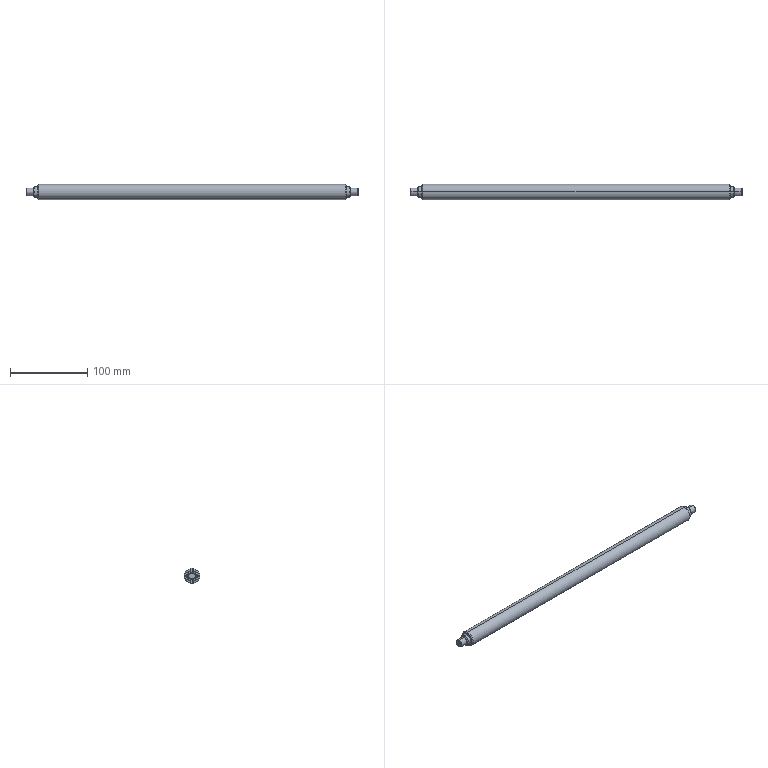Part | STEP file | Flat conveyor mechanism-CN2500x400-111-101 | 1 solid | 28 faces | box 431 x 20 x 20 mm | volume 128796 mm3 | cone 12 | cylinder 10 | plane 6 | commonest cylinder face diameters 10 x4 14 x4 20 x2
STEP:
#1=CARTESIAN_POINT('',(-200.,0.,9.));
#2=VERTEX_POINT('',#1);
#3=CARTESIAN_POINT('',(-200.,0.,-9.));
#4=VERTEX_POINT('',#3);
#5=CARTESIAN_POINT('',(-200.,0.,0.));
#6=DIRECTION('',(-1.,0.,0.));
#7=DIRECTION('',(0.,0.,-1.));
#8=AXIS2_PLACEMENT_3D('',#5,#6,#7);
#9=CIRCLE('',#8,9.);
#10=EDGE_CURVE('',#2,#4,#9,.T.);
#11=ORIENTED_EDGE('',*,*,#10,.F.);
#12=CARTESIAN_POINT('',(-199.,0.,10.));
#13=VERTEX_POINT('',#12);
#14=CARTESIAN_POINT('',(-199.,0.,10.));
#15=DIRECTION('',(0.7071,0.,0.7071));
#16=VECTOR('',#15,1000.);
#17=LINE('',#14,#16);
#18=EDGE_CURVE('',#2,#13,#17,.T.);
#19=ORIENTED_EDGE('',*,*,#18,.T.);
#20=CARTESIAN_POINT('',(-199.,0.,-10.));
#21=VERTEX_POINT('',#20);
#22=CARTESIAN_POINT('',(-199.,0.,0.));
#23=DIRECTION('',(1.,0.,0.));
#24=DIRECTION('',(0.,0.,-1.));
#25=AXIS2_PLACEMENT_3D('',#22,#23,#24);
#26=CIRCLE('',#25,10.);
#27=EDGE_CURVE('',#21,#13,#26,.T.);
#28=ORIENTED_EDGE('',*,*,#27,.F.);
#29=CARTESIAN_POINT('',(-199.,0.,-10.));
#30=DIRECTION('',(0.7071,0.,-0.7071));
#31=VECTOR('',#30,1000.);
#32=LINE('',#29,#31);
#33=EDGE_CURVE('',#4,#21,#32,.T.);
#34=ORIENTED_EDGE('',*,*,#33,.F.);
#35=EDGE_LOOP('',(#11,#19,#28,#34));
#36=FACE_OUTER_BOUND('',#35,.T.);
#37=CARTESIAN_POINT('',(-199.,0.,0.));
#38=DIRECTION('',(1.,0.,0.));
#39=DIRECTION('',(0.,0.,-1.));
#40=AXIS2_PLACEMENT_3D('',#37,#38,#39);
#41=CONICAL_SURFACE('',#40,10.,0.7854);
#42=ADVANCED_FACE('',(#36),#41,.T.);
#43=CARTESIAN_POINT('',(-215.5,0.,4.));
#44=VERTEX_POINT('',#43);
#45=CARTESIAN_POINT('',(-215.5,0.,-4.));
#46=VERTEX_POINT('',#45);
#47=CARTESIAN_POINT('',(-215.5,0.,0.));
#48=DIRECTION('',(-1.,0.,0.));
#49=DIRECTION('',(0.,0.,-1.));
#50=AXIS2_PLACEMENT_3D('',#47,#48,#49);
#51=CIRCLE('',#50,4.);
#52=EDGE_CURVE('',#44,#46,#51,.T.);
#53=ORIENTED_EDGE('',*,*,#52,.F.);
#54=CARTESIAN_POINT('',(-214.5,0.,5.));
#55=VERTEX_POINT('',#54);
#56=CARTESIAN_POINT('',(-214.5,0.,5.));
#57=DIRECTION('',(0.7071,0.,0.7071));
#58=VECTOR('',#57,1000.);
#59=LINE('',#56,#58);
#60=EDGE_CURVE('',#44,#55,#59,.T.);
#61=ORIENTED_EDGE('',*,*,#60,.T.);
#62=CARTESIAN_POINT('',(-214.5,0.,-5.));
#63=VERTEX_POINT('',#62);
#64=CARTESIAN_POINT('',(-214.5,0.,0.));
#65=DIRECTION('',(1.,0.,0.));
#66=DIRECTION('',(0.,0.,-1.));
#67=AXIS2_PLACEMENT_3D('',#64,#65,#66);
#68=CIRCLE('',#67,5.);
#69=EDGE_CURVE('',#63,#55,#68,.T.);
#70=ORIENTED_EDGE('',*,*,#69,.F.);
#71=CARTESIAN_POINT('',(-214.5,0.,-5.));
#72=DIRECTION('',(0.7071,0.,-0.7071));
#73=VECTOR('',#72,1000.);
#74=LINE('',#71,#73);
#75=EDGE_CURVE('',#46,#63,#74,.T.);
#76=ORIENTED_EDGE('',*,*,#75,.F.);
#77=EDGE_LOOP('',(#53,#61,#70,#76));
#78=FACE_OUTER_BOUND('',#77,.T.);
#79=CARTESIAN_POINT('',(-214.5,0.,0.));
#80=DIRECTION('',(1.,0.,0.));
#81=DIRECTION('',(0.,0.,-1.));
#82=AXIS2_PLACEMENT_3D('',#79,#80,#81);
#83=CONICAL_SURFACE('',#82,5.,0.7854);
#84=ADVANCED_FACE('',(#78),#83,.T.);
#85=CARTESIAN_POINT('',(200.,0.,-9.));
#86=VERTEX_POINT('',#85);
#87=CARTESIAN_POINT('',(200.,0.,9.));
#88=VERTEX_POINT('',#87);
#89=CARTESIAN_POINT('',(200.,0.,0.));
#90=DIRECTION('',(1.,0.,0.));
#91=DIRECTION('',(0.,0.,-1.));
#92=AXIS2_PLACEMENT_3D('',#89,#90,#91);
#93=CIRCLE('',#92,9.);
#94=EDGE_CURVE('',#86,#88,#93,.T.);
#95=ORIENTED_EDGE('',*,*,#94,.F.);
#96=CARTESIAN_POINT('',(199.,0.,-10.));
#97=VERTEX_POINT('',#96);
#98=CARTESIAN_POINT('',(200.,0.,-9.));
#99=DIRECTION('',(-0.7071,0.,-0.7071));
#100=VECTOR('',#99,1000.);
#101=LINE('',#98,#100);
#102=EDGE_CURVE('',#86,#97,#101,.T.);
#103=ORIENTED_EDGE('',*,*,#102,.T.);
#104=CARTESIAN_POINT('',(199.,0.,10.));
#105=VERTEX_POINT('',#104);
#106=CARTESIAN_POINT('',(199.,0.,0.));
#107=DIRECTION('',(-1.,0.,0.));
#108=DIRECTION('',(0.,0.,-1.));
#109=AXIS2_PLACEMENT_3D('',#106,#107,#108);
#110=CIRCLE('',#109,10.);
#111=EDGE_CURVE('',#105,#97,#110,.T.);
#112=ORIENTED_EDGE('',*,*,#111,.F.);
#113=CARTESIAN_POINT('',(200.,0.,9.));
#114=DIRECTION('',(-0.7071,0.,0.7071));
#115=VECTOR('',#114,1000.);
#116=LINE('',#113,#115);
#117=EDGE_CURVE('',#88,#105,#116,.T.);
#118=ORIENTED_EDGE('',*,*,#117,.F.);
#119=EDGE_LOOP('',(#95,#103,#112,#118));
#120=FACE_OUTER_BOUND('',#119,.T.);
#121=CARTESIAN_POINT('',(200.,0.,0.));
#122=DIRECTION('',(-1.,0.,0.));
#123=DIRECTION('',(0.,0.,1.));
#124=AXIS2_PLACEMENT_3D('',#121,#122,#123);
#125=CONICAL_SURFACE('',#124,9.,0.7854);
#126=ADVANCED_FACE('',(#120),#125,.T.);
#127=CARTESIAN_POINT('',(215.5,0.,-4.));
#128=VERTEX_POINT('',#127);
#129=CARTESIAN_POINT('',(215.5,0.,4.));
#130=VERTEX_POINT('',#129);
#131=CARTESIAN_POINT('',(215.5,0.,0.));
#132=DIRECTION('',(1.,0.,0.));
#133=DIRECTION('',(0.,0.,-1.));
#134=AXIS2_PLACEMENT_3D('',#131,#132,#133);
#135=CIRCLE('',#134,4.);
#136=EDGE_CURVE('',#128,#130,#135,.T.);
#137=ORIENTED_EDGE('',*,*,#136,.F.);
#138=CARTESIAN_POINT('',(214.5,0.,-5.));
#139=VERTEX_POINT('',#138);
#140=CARTESIAN_POINT('',(215.5,0.,-4.));
#141=DIRECTION('',(-0.7071,0.,-0.7071));
#142=VECTOR('',#141,1000.);
#143=LINE('',#140,#142);
#144=EDGE_CURVE('',#128,#139,#143,.T.);
#145=ORIENTED_EDGE('',*,*,#144,.T.);
#146=CARTESIAN_POINT('',(214.5,0.,5.));
#147=VERTEX_POINT('',#146);
#148=CARTESIAN_POINT('',(214.5,0.,0.));
#149=DIRECTION('',(-1.,0.,0.));
#150=DIRECTION('',(0.,0.,-1.));
#151=AXIS2_PLACEMENT_3D('',#148,#149,#150);
#152=CIRCLE('',#151,5.);
#153=EDGE_CURVE('',#147,#139,#152,.T.);
#154=ORIENTED_EDGE('',*,*,#153,.F.);
#155=CARTESIAN_POINT('',(215.5,0.,4.));
#156=DIRECTION('',(-0.7071,0.,0.7071));
#157=VECTOR('',#156,1000.);
#158=LINE('',#155,#157);
#159=EDGE_CURVE('',#130,#147,#158,.T.);
#160=ORIENTED_EDGE('',*,*,#159,.F.);
#161=EDGE_LOOP('',(#137,#145,#154,#160));
#162=FACE_OUTER_BOUND('',#161,.T.);
#163=CARTESIAN_POINT('',(215.5,0.,0.));
#164=DIRECTION('',(-1.,0.,0.));
#165=DIRECTION('',(0.,0.,1.));
#166=AXIS2_PLACEMENT_3D('',#163,#164,#165);
#167=CONICAL_SURFACE('',#166,4.,0.7854);
#168=ADVANCED_FACE('',(#162),#167,.T.);
#169=CARTESIAN_POINT('',(205.5,0.,-6.));
#170=VERTEX_POINT('',#169);
#171=CARTESIAN_POINT('',(205.5,0.,6.));
#172=VERTEX_POINT('',#171);
#173=CARTESIAN_POINT('',(205.5,0.,0.));
#174=DIRECTION('',(1.,0.,0.));
#175=DIRECTION('',(0.,0.,-1.));
#176=AXIS2_PLACEMENT_3D('',#173,#174,#175);
#177=CIRCLE('',#176,6.);
#178=EDGE_CURVE('',#170,#172,#177,.T.);
#179=ORIENTED_EDGE('',*,*,#178,.F.);
#180=CARTESIAN_POINT('',(204.5,0.,-7.));
#181=VERTEX_POINT('',#180);
#182=CARTESIAN_POINT('',(205.5,0.,-6.));
#183=DIRECTION('',(-0.7071,0.,-0.7071));
#184=VECTOR('',#183,1000.);
#185=LINE('',#182,#184);
#186=EDGE_CURVE('',#170,#181,#185,.T.);
#187=ORIENTED_EDGE('',*,*,#186,.T.);
#188=CARTESIAN_POINT('',(204.5,0.,7.));
#189=VERTEX_POINT('',#188);
#190=CARTESIAN_POINT('',(204.5,0.,0.));
#191=DIRECTION('',(-1.,0.,0.));
#192=DIRECTION('',(0.,0.,-1.));
#193=AXIS2_PLACEMENT_3D('',#190,#191,#192);
#194=CIRCLE('',#193,7.);
#195=EDGE_CURVE('',#189,#181,#194,.T.);
#196=ORIENTED_EDGE('',*,*,#195,.F.);
#197=CARTESIAN_POINT('',(205.5,0.,6.));
#198=DIRECTION('',(-0.7071,0.,0.7071));
#199=VECTOR('',#198,1000.);
#200=LINE('',#197,#199);
#201=EDGE_CURVE('',#172,#189,#200,.T.);
#202=ORIENTED_EDGE('',*,*,#201,.F.);
#203=EDGE_LOOP('',(#179,#187,#196,#202));
#204=FACE_OUTER_BOUND('',#203,.T.);
#205=CARTESIAN_POINT('',(205.5,0.,0.));
#206=DIRECTION('',(-1.,0.,0.));
#207=DIRECTION('',(0.,0.,1.));
#208=AXIS2_PLACEMENT_3D('',#205,#206,#207);
#209=CONICAL_SURFACE('',#208,6.,0.7854);
#210=ADVANCED_FACE('',(#204),#209,.T.);
#211=CARTESIAN_POINT('',(-205.5,0.,6.));
#212=VERTEX_POINT('',#211);
#213=CARTESIAN_POINT('',(-205.5,0.,-6.));
#214=VERTEX_POINT('',#213);
#215=CARTESIAN_POINT('',(-205.5,0.,0.));
#216=DIRECTION('',(-1.,0.,0.));
#217=DIRECTION('',(0.,0.,-1.));
#218=AXIS2_PLACEMENT_3D('',#215,#216,#217);
#219=CIRCLE('',#218,6.);
#220=EDGE_CURVE('',#212,#214,#219,.T.);
#221=ORIENTED_EDGE('',*,*,#220,.F.);
#222=CARTESIAN_POINT('',(-204.5,0.,7.));
#223=VERTEX_POINT('',#222);
#224=CARTESIAN_POINT('',(-204.5,0.,7.));
#225=DIRECTION('',(0.7071,0.,0.7071));
#226=VECTOR('',#225,1000.);
#227=LINE('',#224,#226);
#228=EDGE_CURVE('',#212,#223,#227,.T.);
#229=ORIENTED_EDGE('',*,*,#228,.T.);
#230=CARTESIAN_POINT('',(-204.5,0.,-7.));
#231=VERTEX_POINT('',#230);
#232=CARTESIAN_POINT('',(-204.5,0.,0.));
#233=DIRECTION('',(1.,0.,0.));
#234=DIRECTION('',(0.,0.,-1.));
#235=AXIS2_PLACEMENT_3D('',#232,#233,#234);
#236=CIRCLE('',#235,7.);
#237=EDGE_CURVE('',#231,#223,#236,.T.);
#238=ORIENTED_EDGE('',*,*,#237,.F.);
#239=CARTESIAN_POINT('',(-204.5,0.,-7.));
#240=DIRECTION('',(0.7071,0.,-0.7071));
#241=VECTOR('',#240,1000.);
#242=LINE('',#239,#241);
#243=EDGE_CURVE('',#214,#231,#242,.T.);
#244=ORIENTED_EDGE('',*,*,#243,.F.);
#245=EDGE_LOOP('',(#221,#229,#238,#244));
#246=FACE_OUTER_BOUND('',#245,.T.);
#247=CARTESIAN_POINT('',(-204.5,0.,0.));
#248=DIRECTION('',(1.,0.,0.));
#249=DIRECTION('',(0.,0.,-1.));
#250=AXIS2_PLACEMENT_3D('',#247,#248,#249);
#251=CONICAL_SURFACE('',#250,7.,0.7854);
#252=ADVANCED_FACE('',(#246),#251,.T.);
#253=ORIENTED_EDGE('',*,*,#153,.T.);
#254=CARTESIAN_POINT('',(205.5,0.,-5.));
#255=VERTEX_POINT('',#254);
#256=CARTESIAN_POINT('',(215.5,0.,-5.));
#257=DIRECTION('',(-1.,0.,0.));
#258=VECTOR('',#257,1000.);
#259=LINE('',#256,#258);
#260=EDGE_CURVE('',#139,#255,#259,.T.);
#261=ORIENTED_EDGE('',*,*,#260,.T.);
#262=CARTESIAN_POINT('',(205.5,0.,5.));
#263=VERTEX_POINT('',#262);
#264=CARTESIAN_POINT('',(205.5,0.,0.));
#265=DIRECTION('',(1.,0.,0.));
#266=DIRECTION('',(0.,0.,-1.));
#267=AXIS2_PLACEMENT_3D('',#264,#265,#266);
#268=CIRCLE('',#267,5.);
#269=EDGE_CURVE('',#255,#263,#268,.T.);
#270=ORIENTED_EDGE('',*,*,#269,.T.);
#271=CARTESIAN_POINT('',(215.5,0.,5.));
#272=DIRECTION('',(-1.,0.,0.));
#273=VECTOR('',#272,1000.);
#274=LINE('',#271,#273);
#275=EDGE_CURVE('',#147,#263,#274,.T.);
#276=ORIENTED_EDGE('',*,*,#275,.F.);
#277=EDGE_LOOP('',(#253,#261,#270,#276));
#278=FACE_OUTER_BOUND('',#277,.T.);
#279=CARTESIAN_POINT('',(215.5,0.,0.));
#280=DIRECTION('',(-1.,0.,0.));
#281=DIRECTION('',(0.,0.,1.));
#282=AXIS2_PLACEMENT_3D('',#279,#280,#281);
#283=CYLINDRICAL_SURFACE('',#282,5.);
#284=ADVANCED_FACE('',(#278),#283,.T.);
#285=CARTESIAN_POINT('',(-205.5,0.,-5.));
#286=VERTEX_POINT('',#285);
#287=CARTESIAN_POINT('',(-205.5,0.,5.));
#288=VERTEX_POINT('',#287);
#289=CARTESIAN_POINT('',(-205.5,0.,0.));
#290=DIRECTION('',(1.,0.,0.));
#291=DIRECTION('',(0.,0.,-1.));
#292=AXIS2_PLACEMENT_3D('',#289,#290,#291);
#293=CIRCLE('',#292,5.);
#294=EDGE_CURVE('',#286,#288,#293,.T.);
#295=ORIENTED_EDGE('',*,*,#294,.F.);
#296=CARTESIAN_POINT('',(215.5,0.,-5.));
#297=DIRECTION('',(-1.,0.,0.));
#298=VECTOR('',#297,1000.);
#299=LINE('',#296,#298);
#300=EDGE_CURVE('',#286,#63,#299,.T.);
#301=ORIENTED_EDGE('',*,*,#300,.T.);
#302=ORIENTED_EDGE('',*,*,#69,.T.);
#303=CARTESIAN_POINT('',(215.5,0.,5.));
#304=DIRECTION('',(-1.,0.,0.));
#305=VECTOR('',#304,1000.);
#306=LINE('',#303,#305);
#307=EDGE_CURVE('',#288,#55,#306,.T.);
#308=ORIENTED_EDGE('',*,*,#307,.F.);
#309=EDGE_LOOP('',(#295,#301,#302,#308));
#310=FACE_OUTER_BOUND('',#309,.T.);
#311=CARTESIAN_POINT('',(215.5,0.,0.));
#312=DIRECTION('',(-1.,0.,0.));
#313=DIRECTION('',(0.,0.,1.));
#314=AXIS2_PLACEMENT_3D('',#311,#312,#313);
#315=CYLINDRICAL_SURFACE('',#314,5.);
#316=ADVANCED_FACE('',(#310),#315,.T.);
#317=CARTESIAN_POINT('',(-200.,0.,7.));
#318=VERTEX_POINT('',#317);
#319=CARTESIAN_POINT('',(-200.,0.,-7.));
#320=VERTEX_POINT('',#319);
#321=CARTESIAN_POINT('',(-200.,0.,0.));
#322=DIRECTION('',(-1.,0.,0.));
#323=DIRECTION('',(0.,0.,-1.));
#324=AXIS2_PLACEMENT_3D('',#321,#322,#323);
#325=CIRCLE('',#324,7.);
#326=EDGE_CURVE('',#318,#320,#325,.T.);
#327=ORIENTED_EDGE('',*,*,#326,.T.);
#328=CARTESIAN_POINT('',(205.5,0.,-7.));
#329=DIRECTION('',(-1.,0.,0.));
#330=VECTOR('',#329,1000.);
#331=LINE('',#328,#330);
#332=EDGE_CURVE('',#320,#231,#331,.T.);
#333=ORIENTED_EDGE('',*,*,#332,.T.);
#334=ORIENTED_EDGE('',*,*,#237,.T.);
#335=CARTESIAN_POINT('',(205.5,0.,7.));
#336=DIRECTION('',(-1.,0.,0.));
#337=VECTOR('',#336,1000.);
#338=LINE('',#335,#337);
#339=EDGE_CURVE('',#318,#223,#338,.T.);
#340=ORIENTED_EDGE('',*,*,#339,.F.);
#341=EDGE_LOOP('',(#327,#333,#334,#340));
#342=FACE_OUTER_BOUND('',#341,.T.);
#343=CARTESIAN_POINT('',(205.5,0.,0.));
#344=DIRECTION('',(-1.,0.,0.));
#345=DIRECTION('',(0.,0.,1.));
#346=AXIS2_PLACEMENT_3D('',#343,#344,#345);
#347=CYLINDRICAL_SURFACE('',#346,7.);
#348=ADVANCED_FACE('',(#342),#347,.T.);
#349=ORIENTED_EDGE('',*,*,#195,.T.);
#350=CARTESIAN_POINT('',(200.,0.,-7.));
#351=VERTEX_POINT('',#350);
#352=CARTESIAN_POINT('',(205.5,0.,-7.));
#353=DIRECTION('',(-1.,0.,0.));
#354=VECTOR('',#353,1000.);
#355=LINE('',#352,#354);
#356=EDGE_CURVE('',#181,#351,#355,.T.);
#357=ORIENTED_EDGE('',*,*,#356,.T.);
#358=CARTESIAN_POINT('',(200.,0.,7.));
#359=VERTEX_POINT('',#358);
#360=CARTESIAN_POINT('',(200.,0.,0.));
#361=DIRECTION('',(-1.,0.,0.));
#362=DIRECTION('',(0.,0.,-1.));
#363=AXIS2_PLACEMENT_3D('',#360,#361,#362);
#364=CIRCLE('',#363,7.);
#365=EDGE_CURVE('',#359,#351,#364,.T.);
#366=ORIENTED_EDGE('',*,*,#365,.F.);
#367=CARTESIAN_POINT('',(205.5,0.,7.));
#368=DIRECTION('',(-1.,0.,0.));
#369=VECTOR('',#368,1000.);
#370=LINE('',#367,#369);
#371=EDGE_CURVE('',#189,#359,#370,.T.);
#372=ORIENTED_EDGE('',*,*,#371,.F.);
#373=EDGE_LOOP('',(#349,#357,#366,#372));
#374=FACE_OUTER_BOUND('',#373,.T.);
#375=CARTESIAN_POINT('',(205.5,0.,0.));
#376=DIRECTION('',(-1.,0.,0.));
#377=DIRECTION('',(0.,0.,1.));
#378=AXIS2_PLACEMENT_3D('',#375,#376,#377);
#379=CYLINDRICAL_SURFACE('',#378,7.);
#380=ADVANCED_FACE('',(#374),#379,.T.);
#381=ORIENTED_EDGE('',*,*,#111,.T.);
#382=CARTESIAN_POINT('',(200.,0.,-10.));
#383=DIRECTION('',(-1.,0.,0.));
#384=VECTOR('',#383,1000.);
#385=LINE('',#382,#384);
#386=EDGE_CURVE('',#97,#21,#385,.T.);
#387=ORIENTED_EDGE('',*,*,#386,.T.);
#388=ORIENTED_EDGE('',*,*,#27,.T.);
#389=CARTESIAN_POINT('',(200.,0.,10.));
#390=DIRECTION('',(-1.,0.,0.));
#391=VECTOR('',#390,1000.);
#392=LINE('',#389,#391);
#393=EDGE_CURVE('',#105,#13,#392,.T.);
#394=ORIENTED_EDGE('',*,*,#393,.F.);
#395=EDGE_LOOP('',(#381,#387,#388,#394));
#396=FACE_OUTER_BOUND('',#395,.T.);
#397=CARTESIAN_POINT('',(200.,0.,0.));
#398=DIRECTION('',(-1.,0.,0.));
#399=DIRECTION('',(0.,0.,1.));
#400=AXIS2_PLACEMENT_3D('',#397,#398,#399);
#401=CYLINDRICAL_SURFACE('',#400,10.);
#402=ADVANCED_FACE('',(#396),#401,.T.);
#403=ORIENTED_EDGE('',*,*,#386,.F.);
#404=CARTESIAN_POINT('',(199.,0.,0.));
#405=DIRECTION('',(-1.,0.,0.));
#406=DIRECTION('',(0.,0.,-1.));
#407=AXIS2_PLACEMENT_3D('',#404,#405,#406);
#408=CIRCLE('',#407,10.);
#409=EDGE_CURVE('',#97,#105,#408,.T.);
#410=ORIENTED_EDGE('',*,*,#409,.T.);
#411=ORIENTED_EDGE('',*,*,#393,.T.);
#412=CARTESIAN_POINT('',(-199.,0.,0.));
#413=DIRECTION('',(1.,0.,0.));
#414=DIRECTION('',(0.,0.,-1.));
#415=AXIS2_PLACEMENT_3D('',#412,#413,#414);
#416=CIRCLE('',#415,10.);
#417=EDGE_CURVE('',#13,#21,#416,.T.);
#418=ORIENTED_EDGE('',*,*,#417,.T.);
#419=EDGE_LOOP('',(#403,#410,#411,#418));
#420=FACE_OUTER_BOUND('',#419,.T.);
#421=CARTESIAN_POINT('',(200.,0.,0.));
#422=DIRECTION('',(-1.,0.,0.));
#423=DIRECTION('',(0.,0.,1.));
#424=AXIS2_PLACEMENT_3D('',#421,#422,#423);
#425=CYLINDRICAL_SURFACE('',#424,10.);
#426=ADVANCED_FACE('',(#420),#425,.T.);
#427=CARTESIAN_POINT('',(200.,0.,0.));
#428=DIRECTION('',(1.,0.,0.));
#429=DIRECTION('',(0.,0.,-1.));
#430=AXIS2_PLACEMENT_3D('',#427,#428,#429);
#431=CIRCLE('',#430,9.);
#432=EDGE_CURVE('',#88,#86,#431,.T.);
#433=ORIENTED_EDGE('',*,*,#432,.T.);
#434=ORIENTED_EDGE('',*,*,#94,.T.);
#435=EDGE_LOOP('',(#433,#434));
#436=FACE_OUTER_BOUND('',#435,.T.);
#437=ORIENTED_EDGE('',*,*,#365,.T.);
#438=CARTESIAN_POINT('',(200.,0.,0.));
#439=DIRECTION('',(-1.,0.,0.));
#440=DIRECTION('',(0.,0.,-1.));
#441=AXIS2_PLACEMENT_3D('',#438,#439,#440);
#442=CIRCLE('',#441,7.);
#443=EDGE_CURVE('',#351,#359,#442,.T.);
#444=ORIENTED_EDGE('',*,*,#443,.T.);
#445=EDGE_LOOP('',(#437,#444));
#446=FACE_BOUND('',#445,.T.);
#447=CARTESIAN_POINT('',(200.,0.,0.));
#448=DIRECTION('',(1.,0.,0.));
#449=DIRECTION('',(0.,0.,-1.));
#450=AXIS2_PLACEMENT_3D('',#447,#448,#449);
#451=PLANE('',#450);
#452=ADVANCED_FACE('',(#436,#446),#451,.T.);
#453=CARTESIAN_POINT('',(-200.,0.,0.));
#454=DIRECTION('',(-1.,0.,0.));
#455=DIRECTION('',(0.,0.,-1.));
#456=AXIS2_PLACEMENT_3D('',#453,#454,#455);
#457=CIRCLE('',#456,9.);
#458=EDGE_CURVE('',#4,#2,#457,.T.);
#459=ORIENTED_EDGE('',*,*,#458,.T.);
#460=ORIENTED_EDGE('',*,*,#10,.T.);
#461=EDGE_LOOP('',(#459,#460));
#462=FACE_OUTER_BOUND('',#461,.T.);
#463=ORIENTED_EDGE('',*,*,#326,.F.);
#464=CARTESIAN_POINT('',(-200.,0.,0.));
#465=DIRECTION('',(-1.,0.,0.));
#466=DIRECTION('',(0.,0.,-1.));
#467=AXIS2_PLACEMENT_3D('',#464,#465,#466);
#468=CIRCLE('',#467,7.);
#469=EDGE_CURVE('',#320,#318,#468,.T.);
#470=ORIENTED_EDGE('',*,*,#469,.F.);
#471=EDGE_LOOP('',(#463,#470));
#472=FACE_BOUND('',#471,.T.);
#473=CARTESIAN_POINT('',(-200.,0.,0.));
#474=DIRECTION('',(1.,0.,0.));
#475=DIRECTION('',(0.,0.,-1.));
#476=AXIS2_PLACEMENT_3D('',#473,#474,#475);
#477=PLANE('',#476);
#478=ADVANCED_FACE('',(#462,#472),#477,.F.);
#479=CARTESIAN_POINT('',(205.5,0.,0.));
#480=DIRECTION('',(1.,0.,0.));
#481=DIRECTION('',(0.,0.,-1.));
#482=AXIS2_PLACEMENT_3D('',#479,#480,#481);
#483=CIRCLE('',#482,6.);
#484=EDGE_CURVE('',#172,#170,#483,.T.);
#485=ORIENTED_EDGE('',*,*,#484,.T.);
#486=ORIENTED_EDGE('',*,*,#178,.T.);
#487=EDGE_LOOP('',(#485,#486));
#488=FACE_OUTER_BOUND('',#487,.T.);
#489=CARTESIAN_POINT('',(205.5,0.,0.));
#490=DIRECTION('',(1.,0.,0.));
#491=DIRECTION('',(0.,0.,-1.));
#492=AXIS2_PLACEMENT_3D('',#489,#490,#491);
#493=CIRCLE('',#492,5.);
#494=EDGE_CURVE('',#263,#255,#493,.T.);
#495=ORIENTED_EDGE('',*,*,#494,.F.);
#496=ORIENTED_EDGE('',*,*,#269,.F.);
#497=EDGE_LOOP('',(#495,#496));
#498=FACE_BOUND('',#497,.T.);
#499=CARTESIAN_POINT('',(205.5,0.,0.));
#500=DIRECTION('',(1.,0.,0.));
#501=DIRECTION('',(0.,0.,-1.));
#502=AXIS2_PLACEMENT_3D('',#499,#500,#501);
#503=PLANE('',#502);
#504=ADVANCED_FACE('',(#488,#498),#503,.T.);
#505=ORIENTED_EDGE('',*,*,#356,.F.);
#506=CARTESIAN_POINT('',(204.5,0.,0.));
#507=DIRECTION('',(-1.,0.,0.));
#508=DIRECTION('',(0.,0.,-1.));
#509=AXIS2_PLACEMENT_3D('',#506,#507,#508);
#510=CIRCLE('',#509,7.);
#511=EDGE_CURVE('',#181,#189,#510,.T.);
#512=ORIENTED_EDGE('',*,*,#511,.T.);
#513=ORIENTED_EDGE('',*,*,#371,.T.);
#514=ORIENTED_EDGE('',*,*,#443,.F.);
#515=EDGE_LOOP('',(#505,#512,#513,#514));
#516=FACE_OUTER_BOUND('',#515,.T.);
#517=CARTESIAN_POINT('',(205.5,0.,0.));
#518=DIRECTION('',(-1.,0.,0.));
#519=DIRECTION('',(0.,0.,1.));
#520=AXIS2_PLACEMENT_3D('',#517,#518,#519);
#521=CYLINDRICAL_SURFACE('',#520,7.);
#522=ADVANCED_FACE('',(#516),#521,.T.);
#523=ORIENTED_EDGE('',*,*,#332,.F.);
#524=ORIENTED_EDGE('',*,*,#469,.T.);
#525=ORIENTED_EDGE('',*,*,#339,.T.);
#526=CARTESIAN_POINT('',(-204.5,0.,0.));
#527=DIRECTION('',(1.,0.,0.));
#528=DIRECTION('',(0.,0.,-1.));
#529=AXIS2_PLACEMENT_3D('',#526,#527,#528);
#530=CIRCLE('',#529,7.);
#531=EDGE_CURVE('',#223,#231,#530,.T.);
#532=ORIENTED_EDGE('',*,*,#531,.T.);
#533=EDGE_LOOP('',(#523,#524,#525,#532));
#534=FACE_OUTER_BOUND('',#533,.T.);
#535=CARTESIAN_POINT('',(205.5,0.,0.));
#536=DIRECTION('',(-1.,0.,0.));
#537=DIRECTION('',(0.,0.,1.));
#538=AXIS2_PLACEMENT_3D('',#535,#536,#537);
#539=CYLINDRICAL_SURFACE('',#538,7.);
#540=ADVANCED_FACE('',(#534),#539,.T.);
#541=CARTESIAN_POINT('',(-205.5,0.,0.));
#542=DIRECTION('',(-1.,0.,0.));
#543=DIRECTION('',(0.,0.,-1.));
#544=AXIS2_PLACEMENT_3D('',#541,#542,#543);
#545=CIRCLE('',#544,6.);
#546=EDGE_CURVE('',#214,#212,#545,.T.);
#547=ORIENTED_EDGE('',*,*,#546,.T.);
#548=ORIENTED_EDGE('',*,*,#220,.T.);
#549=EDGE_LOOP('',(#547,#548));
#550=FACE_OUTER_BOUND('',#549,.T.);
#551=CARTESIAN_POINT('',(-205.5,0.,0.));
#552=DIRECTION('',(1.,0.,0.));
#553=DIRECTION('',(0.,0.,-1.));
#554=AXIS2_PLACEMENT_3D('',#551,#552,#553);
#555=CIRCLE('',#554,5.);
#556=EDGE_CURVE('',#288,#286,#555,.T.);
#557=ORIENTED_EDGE('',*,*,#556,.T.);
#558=ORIENTED_EDGE('',*,*,#294,.T.);
#559=EDGE_LOOP('',(#557,#558));
#560=FACE_BOUND('',#559,.T.);
#561=CARTESIAN_POINT('',(-205.5,0.,0.));
#562=DIRECTION('',(1.,0.,0.));
#563=DIRECTION('',(0.,0.,-1.));
#564=AXIS2_PLACEMENT_3D('',#561,#562,#563);
#565=PLANE('',#564);
#566=ADVANCED_FACE('',(#550,#560),#565,.F.);
#567=CARTESIAN_POINT('',(-215.5,0.,0.));
#568=DIRECTION('',(-1.,0.,0.));
#569=DIRECTION('',(0.,0.,-1.));
#570=AXIS2_PLACEMENT_3D('',#567,#568,#569);
#571=CIRCLE('',#570,4.);
#572=EDGE_CURVE('',#46,#44,#571,.T.);
#573=ORIENTED_EDGE('',*,*,#572,.T.);
#574=ORIENTED_EDGE('',*,*,#52,.T.);
#575=EDGE_LOOP('',(#573,#574));
#576=FACE_OUTER_BOUND('',#575,.T.);
#577=CARTESIAN_POINT('',(-215.5,0.,0.));
#578=DIRECTION('',(1.,0.,0.));
#579=DIRECTION('',(0.,0.,-1.));
#580=AXIS2_PLACEMENT_3D('',#577,#578,#579);
#581=PLANE('',#580);
#582=ADVANCED_FACE('',(#576),#581,.F.);
#583=ORIENTED_EDGE('',*,*,#300,.F.);
#584=ORIENTED_EDGE('',*,*,#556,.F.);
#585=ORIENTED_EDGE('',*,*,#307,.T.);
#586=CARTESIAN_POINT('',(-214.5,0.,0.));
#587=DIRECTION('',(1.,0.,0.));
#588=DIRECTION('',(0.,0.,-1.));
#589=AXIS2_PLACEMENT_3D('',#586,#587,#588);
#590=CIRCLE('',#589,5.);
#591=EDGE_CURVE('',#55,#63,#590,.T.);
#592=ORIENTED_EDGE('',*,*,#591,.T.);
#593=EDGE_LOOP('',(#583,#584,#585,#592));
#594=FACE_OUTER_BOUND('',#593,.T.);
#595=CARTESIAN_POINT('',(215.5,0.,0.));
#596=DIRECTION('',(-1.,0.,0.));
#597=DIRECTION('',(0.,0.,1.));
#598=AXIS2_PLACEMENT_3D('',#595,#596,#597);
#599=CYLINDRICAL_SURFACE('',#598,5.);
#600=ADVANCED_FACE('',(#594),#599,.T.);
#601=CARTESIAN_POINT('',(215.5,0.,0.));
#602=DIRECTION('',(1.,0.,0.));
#603=DIRECTION('',(0.,0.,-1.));
#604=AXIS2_PLACEMENT_3D('',#601,#602,#603);
#605=CIRCLE('',#604,4.);
#606=EDGE_CURVE('',#130,#128,#605,.T.);
#607=ORIENTED_EDGE('',*,*,#606,.T.);
#608=ORIENTED_EDGE('',*,*,#136,.T.);
#609=EDGE_LOOP('',(#607,#608));
#610=FACE_OUTER_BOUND('',#609,.T.);
#611=CARTESIAN_POINT('',(215.5,0.,0.));
#612=DIRECTION('',(1.,0.,0.));
#613=DIRECTION('',(0.,0.,-1.));
#614=AXIS2_PLACEMENT_3D('',#611,#612,#613);
#615=PLANE('',#614);
#616=ADVANCED_FACE('',(#610),#615,.T.);
#617=ORIENTED_EDGE('',*,*,#260,.F.);
#618=CARTESIAN_POINT('',(214.5,0.,0.));
#619=DIRECTION('',(-1.,0.,0.));
#620=DIRECTION('',(0.,0.,-1.));
#621=AXIS2_PLACEMENT_3D('',#618,#619,#620);
#622=CIRCLE('',#621,5.);
#623=EDGE_CURVE('',#139,#147,#622,.T.);
#624=ORIENTED_EDGE('',*,*,#623,.T.);
#625=ORIENTED_EDGE('',*,*,#275,.T.);
#626=ORIENTED_EDGE('',*,*,#494,.T.);
#627=EDGE_LOOP('',(#617,#624,#625,#626));
#628=FACE_OUTER_BOUND('',#627,.T.);
#629=CARTESIAN_POINT('',(215.5,0.,0.));
#630=DIRECTION('',(-1.,0.,0.));
#631=DIRECTION('',(0.,0.,1.));
#632=AXIS2_PLACEMENT_3D('',#629,#630,#631);
#633=CYLINDRICAL_SURFACE('',#632,5.);
#634=ADVANCED_FACE('',(#628),#633,.T.);
#635=ORIENTED_EDGE('',*,*,#228,.F.);
#636=ORIENTED_EDGE('',*,*,#546,.F.);
#637=ORIENTED_EDGE('',*,*,#243,.T.);
#638=ORIENTED_EDGE('',*,*,#531,.F.);
#639=EDGE_LOOP('',(#635,#636,#637,#638));
#640=FACE_OUTER_BOUND('',#639,.T.);
#641=CARTESIAN_POINT('',(-204.5,0.,0.));
#642=DIRECTION('',(1.,0.,0.));
#643=DIRECTION('',(0.,0.,-1.));
#644=AXIS2_PLACEMENT_3D('',#641,#642,#643);
#645=CONICAL_SURFACE('',#644,7.,0.7854);
#646=ADVANCED_FACE('',(#640),#645,.T.);
#647=ORIENTED_EDGE('',*,*,#186,.F.);
#648=ORIENTED_EDGE('',*,*,#484,.F.);
#649=ORIENTED_EDGE('',*,*,#201,.T.);
#650=ORIENTED_EDGE('',*,*,#511,.F.);
#651=EDGE_LOOP('',(#647,#648,#649,#650));
#652=FACE_OUTER_BOUND('',#651,.T.);
#653=CARTESIAN_POINT('',(205.5,0.,0.));
#654=DIRECTION('',(-1.,0.,0.));
#655=DIRECTION('',(0.,0.,1.));
#656=AXIS2_PLACEMENT_3D('',#653,#654,#655);
#657=CONICAL_SURFACE('',#656,6.,0.7854);
#658=ADVANCED_FACE('',(#652),#657,.T.);
#659=ORIENTED_EDGE('',*,*,#144,.F.);
#660=ORIENTED_EDGE('',*,*,#606,.F.);
#661=ORIENTED_EDGE('',*,*,#159,.T.);
#662=ORIENTED_EDGE('',*,*,#623,.F.);
#663=EDGE_LOOP('',(#659,#660,#661,#662));
#664=FACE_OUTER_BOUND('',#663,.T.);
#665=CARTESIAN_POINT('',(215.5,0.,0.));
#666=DIRECTION('',(-1.,0.,0.));
#667=DIRECTION('',(0.,0.,1.));
#668=AXIS2_PLACEMENT_3D('',#665,#666,#667);
#669=CONICAL_SURFACE('',#668,4.,0.7854);
#670=ADVANCED_FACE('',(#664),#669,.T.);
#671=ORIENTED_EDGE('',*,*,#102,.F.);
#672=ORIENTED_EDGE('',*,*,#432,.F.);
#673=ORIENTED_EDGE('',*,*,#117,.T.);
#674=ORIENTED_EDGE('',*,*,#409,.F.);
#675=EDGE_LOOP('',(#671,#672,#673,#674));
#676=FACE_OUTER_BOUND('',#675,.T.);
#677=CARTESIAN_POINT('',(200.,0.,0.));
#678=DIRECTION('',(-1.,0.,0.));
#679=DIRECTION('',(0.,0.,1.));
#680=AXIS2_PLACEMENT_3D('',#677,#678,#679);
#681=CONICAL_SURFACE('',#680,9.,0.7854);
#682=ADVANCED_FACE('',(#676),#681,.T.);
#683=ORIENTED_EDGE('',*,*,#60,.F.);
#684=ORIENTED_EDGE('',*,*,#572,.F.);
#685=ORIENTED_EDGE('',*,*,#75,.T.);
#686=ORIENTED_EDGE('',*,*,#591,.F.);
#687=EDGE_LOOP('',(#683,#684,#685,#686));
#688=FACE_OUTER_BOUND('',#687,.T.);
#689=CARTESIAN_POINT('',(-214.5,0.,0.));
#690=DIRECTION('',(1.,0.,0.));
#691=DIRECTION('',(0.,0.,-1.));
#692=AXIS2_PLACEMENT_3D('',#689,#690,#691);
#693=CONICAL_SURFACE('',#692,5.,0.7854);
#694=ADVANCED_FACE('',(#688),#693,.T.);
#695=ORIENTED_EDGE('',*,*,#18,.F.);
#696=ORIENTED_EDGE('',*,*,#458,.F.);
#697=ORIENTED_EDGE('',*,*,#33,.T.);
#698=ORIENTED_EDGE('',*,*,#417,.F.);
#699=EDGE_LOOP('',(#695,#696,#697,#698));
#700=FACE_OUTER_BOUND('',#699,.T.);
#701=CARTESIAN_POINT('',(-199.,0.,0.));
#702=DIRECTION('',(1.,0.,0.));
#703=DIRECTION('',(0.,0.,-1.));
#704=AXIS2_PLACEMENT_3D('',#701,#702,#703);
#705=CONICAL_SURFACE('',#704,10.,0.7854);
#706=ADVANCED_FACE('',(#700),#705,.T.);
#707=CLOSED_SHELL('',(#42,#84,#126,#168,#210,#252,#284,#316,#348,#380,#402,#426,#452,#478,#504,#522,#540,#566,#582,#600,#616,#634,#646,#658,#670,#682,#694,#706));
#708=MANIFOLD_SOLID_BREP('',#707);
#709=CARTESIAN_POINT('',(0.,0.,0.));
#710=DIRECTION('',(0.,0.,1.));
#711=DIRECTION('',(1.,0.,0.));
#712=AXIS2_PLACEMENT_3D('',#709,#710,#711);
#713=(LENGTH_UNIT()NAMED_UNIT(*)SI_UNIT(.MILLI.,.METRE.));
#714=UNCERTAINTY_MEASURE_WITH_UNIT(LENGTH_MEASURE(0.00001),#713,'','');
#715=(NAMED_UNIT(*)PLANE_ANGLE_UNIT()SI_UNIT($,.RADIAN.));
#716=(NAMED_UNIT(*)SI_UNIT($,.STERADIAN.)SOLID_ANGLE_UNIT());
#717=(GEOMETRIC_REPRESENTATION_CONTEXT(3)GLOBAL_UNCERTAINTY_ASSIGNED_CONTEXT((#714))GLOBAL_UNIT_ASSIGNED_CONTEXT((#713,#715,#716))REPRESENTATION_CONTEXT('',''));
#718=ADVANCED_BREP_SHAPE_REPRESENTATION('',(#708,#712),#717);